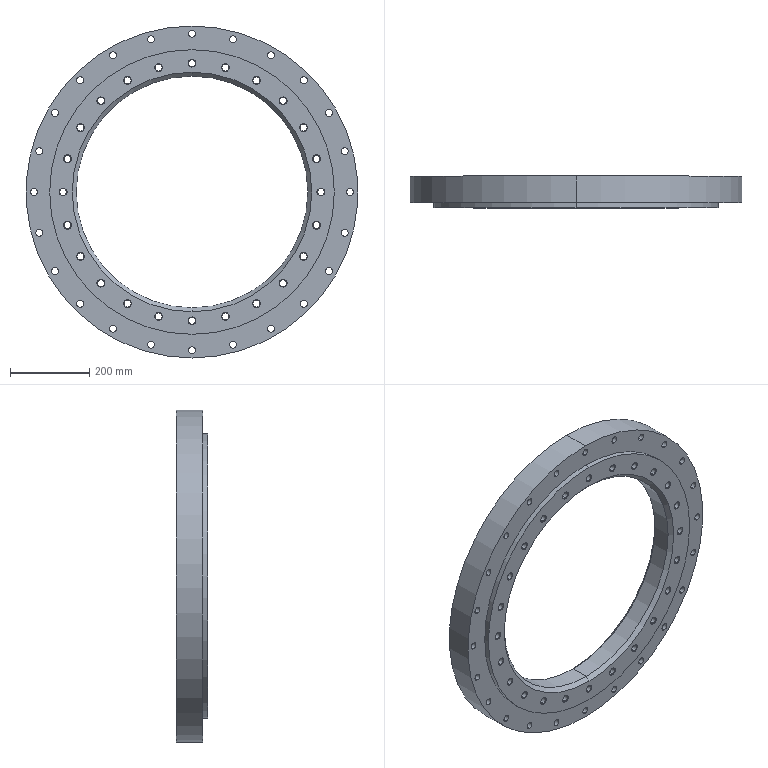Part | SolidWorks | features ICE 3, HoleWzd 2, Chamfer 1, Extrusion 1 | 1 solid | 208 faces | box 840 x 80 x 840 mm | volume 18083089 mm3 | cylinder 104 | cone 100 | plane 4 | commonest cylinder face diameters 17.5 x96 586 x2 720 x2 721 x2 840 x2